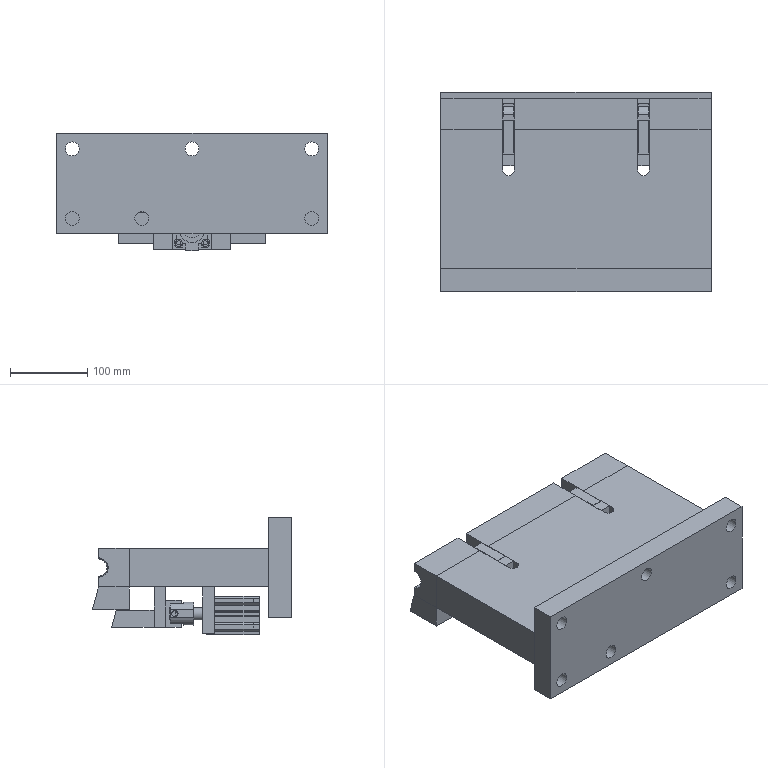Part | NX | features MOVE_FACE 4, lower clamp 4, lower clamp stand 3, CDQ2B32-35DM_CQ2 SnapRing_32 2, CDQ2B32-35DM_CQ22031Rods_32M 2, CDQ2B32-35DM_CQ2Tube_32B 2, CDQ2B32-35DM_RodEndNuts_M14X1.5 2, ISO 4762 M8 x 30 --- 30N_ISO 4762 M8 x 30 --- 30N 2, ejector support 2, lower clamp support 2, pipe ejector 2, pipe injector 2, pneumatic support 2, pneumatic support1 2, pneumatic support2 2 | 30 solids | 680 faces | box 350 x 257.905 x 151.7 mm | volume 5787641 mm3 | plane 427 | cylinder 128 | spline 67 | cone 58 | commonest cylinder face diameters 9 x22 15 x16 8 x14 13 x12 6 x7 5.5 x6